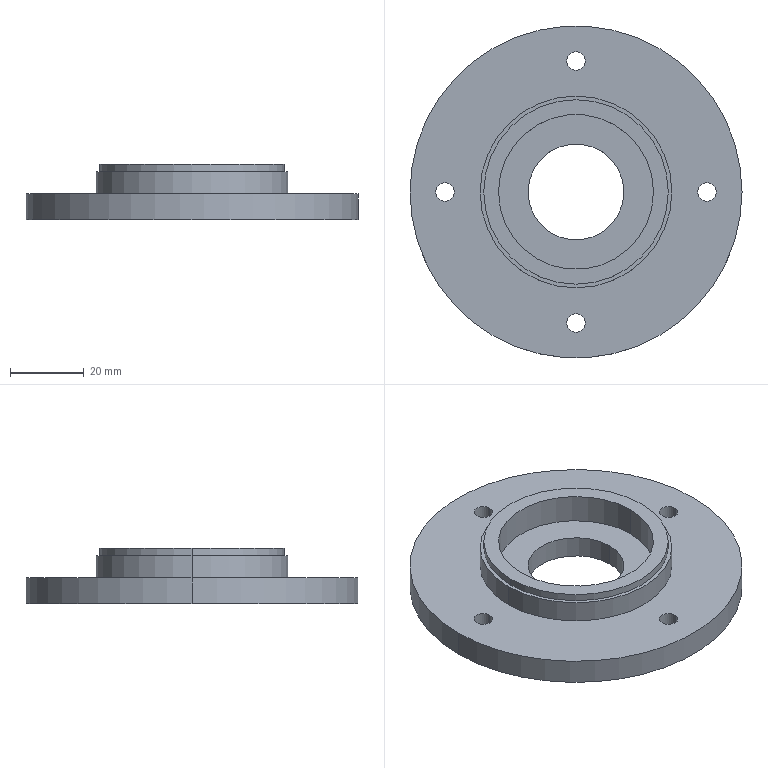Part | SolidWorks | features BaseBody 1 | 1 solid | 28 faces | box 90 x 90 x 15 mm | volume 44792 mm3 | cylinder 18 | plane 6 | torus 4 | commonest cylinder face diameters 5 x8 26 x2 42 x2 50 x2 52 x2 90 x2
STEP:
#1=CARTESIAN_POINT('',(-22.5,0.,0.5));
#2=VERTEX_POINT('',#1);
#3=CARTESIAN_POINT('',(22.5,0.,0.5));
#4=VERTEX_POINT('',#3);
#5=CARTESIAN_POINT('',(0.,0.,0.5));
#6=DIRECTION('',(0.,0.,1.));
#7=DIRECTION('',(1.,0.,0.));
#8=AXIS2_PLACEMENT_3D('',#5,#6,#7);
#9=CIRCLE('',#8,22.5);
#10=EDGE_CURVE('',#2,#4,#9,.T.);
#11=ORIENTED_EDGE('',*,*,#10,.F.);
#12=CARTESIAN_POINT('',(-22.,0.,1.));
#13=VERTEX_POINT('',#12);
#14=CARTESIAN_POINT('',(-22.,0.,0.5));
#15=DIRECTION('',(0.,1.,0.));
#16=DIRECTION('',(-1.,0.,0.));
#17=AXIS2_PLACEMENT_3D('',#14,#15,#16);
#18=CIRCLE('',#17,0.5);
#19=EDGE_CURVE('',#2,#13,#18,.T.);
#20=ORIENTED_EDGE('',*,*,#19,.T.);
#21=CARTESIAN_POINT('',(22.,0.,1.));
#22=VERTEX_POINT('',#21);
#23=CARTESIAN_POINT('',(0.,0.,1.));
#24=DIRECTION('',(0.,0.,1.));
#25=DIRECTION('',(1.,0.,0.));
#26=AXIS2_PLACEMENT_3D('',#23,#24,#25);
#27=CIRCLE('',#26,22.);
#28=EDGE_CURVE('',#13,#22,#27,.T.);
#29=ORIENTED_EDGE('',*,*,#28,.T.);
#30=CARTESIAN_POINT('',(22.,0.,0.5));
#31=DIRECTION('',(0.,-1.,0.));
#32=DIRECTION('',(0.,0.,-1.));
#33=AXIS2_PLACEMENT_3D('',#30,#31,#32);
#34=CIRCLE('',#33,0.5);
#35=EDGE_CURVE('',#4,#22,#34,.T.);
#36=ORIENTED_EDGE('',*,*,#35,.F.);
#37=EDGE_LOOP('',(#11,#20,#29,#36));
#38=FACE_OUTER_BOUND('',#37,.T.);
#39=CARTESIAN_POINT('',(0.,0.,0.5));
#40=DIRECTION('',(0.,0.,1.));
#41=DIRECTION('',(1.,0.,0.));
#42=AXIS2_PLACEMENT_3D('',#39,#40,#41);
#43=TOROIDAL_SURFACE('',#42,22.,0.5);
#44=ADVANCED_FACE('',(#38),#43,.F.);
#45=CARTESIAN_POINT('',(0.,0.,0.5));
#46=DIRECTION('',(0.,0.,1.));
#47=DIRECTION('',(1.,0.,0.));
#48=AXIS2_PLACEMENT_3D('',#45,#46,#47);
#49=CIRCLE('',#48,22.5);
#50=EDGE_CURVE('',#4,#2,#49,.T.);
#51=ORIENTED_EDGE('',*,*,#50,.T.);
#52=CARTESIAN_POINT('',(-23.,0.,0.));
#53=VERTEX_POINT('',#52);
#54=CARTESIAN_POINT('',(-23.,0.,0.5));
#55=DIRECTION('',(0.,1.,0.));
#56=DIRECTION('',(-1.,0.,0.));
#57=AXIS2_PLACEMENT_3D('',#54,#55,#56);
#58=CIRCLE('',#57,0.5);
#59=EDGE_CURVE('',#2,#53,#58,.T.);
#60=ORIENTED_EDGE('',*,*,#59,.T.);
#61=CARTESIAN_POINT('',(23.,0.,0.));
#62=VERTEX_POINT('',#61);
#63=CARTESIAN_POINT('',(0.,0.,0.));
#64=DIRECTION('',(0.,0.,-1.));
#65=DIRECTION('',(1.,0.,0.));
#66=AXIS2_PLACEMENT_3D('',#63,#64,#65);
#67=CIRCLE('',#66,23.);
#68=EDGE_CURVE('',#53,#62,#67,.T.);
#69=ORIENTED_EDGE('',*,*,#68,.T.);
#70=CARTESIAN_POINT('',(23.,0.,0.5));
#71=DIRECTION('',(0.,-1.,0.));
#72=DIRECTION('',(0.,0.,-1.));
#73=AXIS2_PLACEMENT_3D('',#70,#71,#72);
#74=CIRCLE('',#73,0.5);
#75=EDGE_CURVE('',#4,#62,#74,.T.);
#76=ORIENTED_EDGE('',*,*,#75,.F.);
#77=EDGE_LOOP('',(#51,#60,#69,#76));
#78=FACE_OUTER_BOUND('',#77,.T.);
#79=CARTESIAN_POINT('',(0.,0.,0.5));
#80=DIRECTION('',(0.,0.,1.));
#81=DIRECTION('',(1.,0.,0.));
#82=AXIS2_PLACEMENT_3D('',#79,#80,#81);
#83=TOROIDAL_SURFACE('',#82,23.,0.5);
#84=ADVANCED_FACE('',(#78),#83,.T.);
#85=CARTESIAN_POINT('',(33.,0.,7.));
#86=VERTEX_POINT('',#85);
#87=CARTESIAN_POINT('',(38.,0.,7.));
#88=VERTEX_POINT('',#87);
#89=CARTESIAN_POINT('',(35.5,0.,7.));
#90=DIRECTION('',(0.,0.,-1.));
#91=DIRECTION('',(1.,0.,0.));
#92=AXIS2_PLACEMENT_3D('',#89,#90,#91);
#93=CIRCLE('',#92,2.5);
#94=EDGE_CURVE('',#86,#88,#93,.T.);
#95=ORIENTED_EDGE('',*,*,#94,.F.);
#96=CARTESIAN_POINT('',(33.,0.,0.));
#97=VERTEX_POINT('',#96);
#98=CARTESIAN_POINT('',(33.,0.,0.));
#99=DIRECTION('',(0.,0.,-1.));
#100=VECTOR('',#99,1000.);
#101=LINE('',#98,#100);
#102=EDGE_CURVE('',#86,#97,#101,.T.);
#103=ORIENTED_EDGE('',*,*,#102,.T.);
#104=CARTESIAN_POINT('',(38.,0.,0.));
#105=VERTEX_POINT('',#104);
#106=CARTESIAN_POINT('',(35.5,0.,0.));
#107=DIRECTION('',(0.,0.,1.));
#108=DIRECTION('',(1.,0.,0.));
#109=AXIS2_PLACEMENT_3D('',#106,#107,#108);
#110=CIRCLE('',#109,2.5);
#111=EDGE_CURVE('',#105,#97,#110,.T.);
#112=ORIENTED_EDGE('',*,*,#111,.F.);
#113=CARTESIAN_POINT('',(38.,0.,0.));
#114=DIRECTION('',(0.,0.,-1.));
#115=VECTOR('',#114,1000.);
#116=LINE('',#113,#115);
#117=EDGE_CURVE('',#88,#105,#116,.T.);
#118=ORIENTED_EDGE('',*,*,#117,.F.);
#119=EDGE_LOOP('',(#95,#103,#112,#118));
#120=FACE_OUTER_BOUND('',#119,.T.);
#121=CARTESIAN_POINT('',(35.5,0.,0.));
#122=DIRECTION('',(0.,0.,-1.));
#123=DIRECTION('',(1.,0.,0.));
#124=AXIS2_PLACEMENT_3D('',#121,#122,#123);
#125=CYLINDRICAL_SURFACE('',#124,2.5);
#126=ADVANCED_FACE('',(#120),#125,.F.);
#127=CARTESIAN_POINT('',(-2.5,-35.5,7.));
#128=VERTEX_POINT('',#127);
#129=CARTESIAN_POINT('',(2.5,-35.5,7.));
#130=VERTEX_POINT('',#129);
#131=CARTESIAN_POINT('',(0.,-35.5,7.));
#132=DIRECTION('',(0.,0.,-1.));
#133=DIRECTION('',(1.,0.,0.));
#134=AXIS2_PLACEMENT_3D('',#131,#132,#133);
#135=CIRCLE('',#134,2.5);
#136=EDGE_CURVE('',#128,#130,#135,.T.);
#137=ORIENTED_EDGE('',*,*,#136,.F.);
#138=CARTESIAN_POINT('',(-2.5,-35.5,0.));
#139=VERTEX_POINT('',#138);
#140=CARTESIAN_POINT('',(-2.5,-35.5,0.));
#141=DIRECTION('',(0.,0.,-1.));
#142=VECTOR('',#141,1000.);
#143=LINE('',#140,#142);
#144=EDGE_CURVE('',#128,#139,#143,.T.);
#145=ORIENTED_EDGE('',*,*,#144,.T.);
#146=CARTESIAN_POINT('',(2.5,-35.5,0.));
#147=VERTEX_POINT('',#146);
#148=CARTESIAN_POINT('',(0.,-35.5,0.));
#149=DIRECTION('',(0.,0.,1.));
#150=DIRECTION('',(1.,0.,0.));
#151=AXIS2_PLACEMENT_3D('',#148,#149,#150);
#152=CIRCLE('',#151,2.5);
#153=EDGE_CURVE('',#147,#139,#152,.T.);
#154=ORIENTED_EDGE('',*,*,#153,.F.);
#155=CARTESIAN_POINT('',(2.5,-35.5,0.));
#156=DIRECTION('',(0.,0.,-1.));
#157=VECTOR('',#156,1000.);
#158=LINE('',#155,#157);
#159=EDGE_CURVE('',#130,#147,#158,.T.);
#160=ORIENTED_EDGE('',*,*,#159,.F.);
#161=EDGE_LOOP('',(#137,#145,#154,#160));
#162=FACE_OUTER_BOUND('',#161,.T.);
#163=CARTESIAN_POINT('',(0.,-35.5,0.));
#164=DIRECTION('',(0.,0.,-1.));
#165=DIRECTION('',(1.,0.,0.));
#166=AXIS2_PLACEMENT_3D('',#163,#164,#165);
#167=CYLINDRICAL_SURFACE('',#166,2.5);
#168=ADVANCED_FACE('',(#162),#167,.F.);
#169=CARTESIAN_POINT('',(-38.,0.,7.));
#170=VERTEX_POINT('',#169);
#171=CARTESIAN_POINT('',(-33.,0.,7.));
#172=VERTEX_POINT('',#171);
#173=CARTESIAN_POINT('',(-35.5,0.,7.));
#174=DIRECTION('',(0.,0.,-1.));
#175=DIRECTION('',(1.,0.,0.));
#176=AXIS2_PLACEMENT_3D('',#173,#174,#175);
#177=CIRCLE('',#176,2.5);
#178=EDGE_CURVE('',#170,#172,#177,.T.);
#179=ORIENTED_EDGE('',*,*,#178,.F.);
#180=CARTESIAN_POINT('',(-38.,0.,0.));
#181=VERTEX_POINT('',#180);
#182=CARTESIAN_POINT('',(-38.,0.,0.));
#183=DIRECTION('',(0.,0.,-1.));
#184=VECTOR('',#183,1000.);
#185=LINE('',#182,#184);
#186=EDGE_CURVE('',#170,#181,#185,.T.);
#187=ORIENTED_EDGE('',*,*,#186,.T.);
#188=CARTESIAN_POINT('',(-33.,0.,0.));
#189=VERTEX_POINT('',#188);
#190=CARTESIAN_POINT('',(-35.5,0.,0.));
#191=DIRECTION('',(0.,0.,1.));
#192=DIRECTION('',(1.,0.,0.));
#193=AXIS2_PLACEMENT_3D('',#190,#191,#192);
#194=CIRCLE('',#193,2.5);
#195=EDGE_CURVE('',#189,#181,#194,.T.);
#196=ORIENTED_EDGE('',*,*,#195,.F.);
#197=CARTESIAN_POINT('',(-33.,0.,0.));
#198=DIRECTION('',(0.,0.,-1.));
#199=VECTOR('',#198,1000.);
#200=LINE('',#197,#199);
#201=EDGE_CURVE('',#172,#189,#200,.T.);
#202=ORIENTED_EDGE('',*,*,#201,.F.);
#203=EDGE_LOOP('',(#179,#187,#196,#202));
#204=FACE_OUTER_BOUND('',#203,.T.);
#205=CARTESIAN_POINT('',(-35.5,0.,0.));
#206=DIRECTION('',(0.,0.,-1.));
#207=DIRECTION('',(1.,0.,0.));
#208=AXIS2_PLACEMENT_3D('',#205,#206,#207);
#209=CYLINDRICAL_SURFACE('',#208,2.5);
#210=ADVANCED_FACE('',(#204),#209,.F.);
#211=CARTESIAN_POINT('',(-2.5,35.5,7.));
#212=VERTEX_POINT('',#211);
#213=CARTESIAN_POINT('',(2.5,35.5,7.));
#214=VERTEX_POINT('',#213);
#215=CARTESIAN_POINT('',(0.,35.5,7.));
#216=DIRECTION('',(0.,0.,-1.));
#217=DIRECTION('',(1.,0.,0.));
#218=AXIS2_PLACEMENT_3D('',#215,#216,#217);
#219=CIRCLE('',#218,2.5);
#220=EDGE_CURVE('',#212,#214,#219,.T.);
#221=ORIENTED_EDGE('',*,*,#220,.F.);
#222=CARTESIAN_POINT('',(-2.5,35.5,0.));
#223=VERTEX_POINT('',#222);
#224=CARTESIAN_POINT('',(-2.5,35.5,0.));
#225=DIRECTION('',(0.,0.,-1.));
#226=VECTOR('',#225,1000.);
#227=LINE('',#224,#226);
#228=EDGE_CURVE('',#212,#223,#227,.T.);
#229=ORIENTED_EDGE('',*,*,#228,.T.);
#230=CARTESIAN_POINT('',(2.5,35.5,0.));
#231=VERTEX_POINT('',#230);
#232=CARTESIAN_POINT('',(0.,35.5,0.));
#233=DIRECTION('',(0.,0.,1.));
#234=DIRECTION('',(1.,0.,0.));
#235=AXIS2_PLACEMENT_3D('',#232,#233,#234);
#236=CIRCLE('',#235,2.5);
#237=EDGE_CURVE('',#231,#223,#236,.T.);
#238=ORIENTED_EDGE('',*,*,#237,.F.);
#239=CARTESIAN_POINT('',(2.5,35.5,0.));
#240=DIRECTION('',(0.,0.,-1.));
#241=VECTOR('',#240,1000.);
#242=LINE('',#239,#241);
#243=EDGE_CURVE('',#214,#231,#242,.T.);
#244=ORIENTED_EDGE('',*,*,#243,.F.);
#245=EDGE_LOOP('',(#221,#229,#238,#244));
#246=FACE_OUTER_BOUND('',#245,.T.);
#247=CARTESIAN_POINT('',(0.,35.5,0.));
#248=DIRECTION('',(0.,0.,-1.));
#249=DIRECTION('',(1.,0.,0.));
#250=AXIS2_PLACEMENT_3D('',#247,#248,#249);
#251=CYLINDRICAL_SURFACE('',#250,2.5);
#252=ADVANCED_FACE('',(#246),#251,.F.);
#253=CARTESIAN_POINT('',(-13.,0.,1.));
#254=VERTEX_POINT('',#253);
#255=CARTESIAN_POINT('',(13.,0.,1.));
#256=VERTEX_POINT('',#255);
#257=CARTESIAN_POINT('',(0.,0.,1.));
#258=DIRECTION('',(0.,0.,-1.));
#259=DIRECTION('',(-1.,0.,0.));
#260=AXIS2_PLACEMENT_3D('',#257,#258,#259);
#261=CIRCLE('',#260,13.);
#262=EDGE_CURVE('',#254,#256,#261,.T.);
#263=ORIENTED_EDGE('',*,*,#262,.T.);
#264=CARTESIAN_POINT('',(13.,0.,7.));
#265=VERTEX_POINT('',#264);
#266=CARTESIAN_POINT('',(13.,0.,7.));
#267=DIRECTION('',(0.,0.,1.));
#268=VECTOR('',#267,1000.);
#269=LINE('',#266,#268);
#270=EDGE_CURVE('',#256,#265,#269,.T.);
#271=ORIENTED_EDGE('',*,*,#270,.T.);
#272=CARTESIAN_POINT('',(-13.,0.,7.));
#273=VERTEX_POINT('',#272);
#274=CARTESIAN_POINT('',(0.,0.,7.));
#275=DIRECTION('',(0.,0.,-1.));
#276=DIRECTION('',(-1.,0.,0.));
#277=AXIS2_PLACEMENT_3D('',#274,#275,#276);
#278=CIRCLE('',#277,13.);
#279=EDGE_CURVE('',#273,#265,#278,.T.);
#280=ORIENTED_EDGE('',*,*,#279,.F.);
#281=CARTESIAN_POINT('',(-13.,0.,7.));
#282=DIRECTION('',(0.,0.,1.));
#283=VECTOR('',#282,1000.);
#284=LINE('',#281,#283);
#285=EDGE_CURVE('',#254,#273,#284,.T.);
#286=ORIENTED_EDGE('',*,*,#285,.F.);
#287=EDGE_LOOP('',(#263,#271,#280,#286));
#288=FACE_OUTER_BOUND('',#287,.T.);
#289=CARTESIAN_POINT('',(0.,0.,7.));
#290=DIRECTION('',(0.,0.,1.));
#291=DIRECTION('',(-1.,0.,0.));
#292=AXIS2_PLACEMENT_3D('',#289,#290,#291);
#293=CYLINDRICAL_SURFACE('',#292,13.);
#294=ADVANCED_FACE('',(#288),#293,.F.);
#295=CARTESIAN_POINT('',(-25.,0.,13.));
#296=VERTEX_POINT('',#295);
#297=CARTESIAN_POINT('',(25.,0.,13.));
#298=VERTEX_POINT('',#297);
#299=CARTESIAN_POINT('',(0.,0.,13.));
#300=DIRECTION('',(0.,0.,1.));
#301=DIRECTION('',(-1.,0.,0.));
#302=AXIS2_PLACEMENT_3D('',#299,#300,#301);
#303=CIRCLE('',#302,25.);
#304=EDGE_CURVE('',#296,#298,#303,.T.);
#305=ORIENTED_EDGE('',*,*,#304,.T.);
#306=CARTESIAN_POINT('',(25.,0.,15.));
#307=VERTEX_POINT('',#306);
#308=CARTESIAN_POINT('',(25.,0.,15.));
#309=DIRECTION('',(0.,0.,1.));
#310=VECTOR('',#309,1000.);
#311=LINE('',#308,#310);
#312=EDGE_CURVE('',#298,#307,#311,.T.);
#313=ORIENTED_EDGE('',*,*,#312,.T.);
#314=CARTESIAN_POINT('',(-25.,0.,15.));
#315=VERTEX_POINT('',#314);
#316=CARTESIAN_POINT('',(0.,0.,15.));
#317=DIRECTION('',(0.,0.,1.));
#318=DIRECTION('',(-1.,0.,0.));
#319=AXIS2_PLACEMENT_3D('',#316,#317,#318);
#320=CIRCLE('',#319,25.);
#321=EDGE_CURVE('',#315,#307,#320,.T.);
#322=ORIENTED_EDGE('',*,*,#321,.F.);
#323=CARTESIAN_POINT('',(-25.,0.,15.));
#324=DIRECTION('',(0.,0.,1.));
#325=VECTOR('',#324,1000.);
#326=LINE('',#323,#325);
#327=EDGE_CURVE('',#296,#315,#326,.T.);
#328=ORIENTED_EDGE('',*,*,#327,.F.);
#329=EDGE_LOOP('',(#305,#313,#322,#328));
#330=FACE_OUTER_BOUND('',#329,.T.);
#331=CARTESIAN_POINT('',(0.,0.,15.));
#332=DIRECTION('',(0.,0.,1.));
#333=DIRECTION('',(-1.,0.,0.));
#334=AXIS2_PLACEMENT_3D('',#331,#332,#333);
#335=CYLINDRICAL_SURFACE('',#334,25.);
#336=ADVANCED_FACE('',(#330),#335,.T.);
#337=CARTESIAN_POINT('',(21.,0.,15.));
#338=VERTEX_POINT('',#337);
#339=CARTESIAN_POINT('',(-21.,0.,15.));
#340=VERTEX_POINT('',#339);
#341=CARTESIAN_POINT('',(0.,0.,15.));
#342=DIRECTION('',(0.,0.,-1.));
#343=DIRECTION('',(-1.,0.,0.));
#344=AXIS2_PLACEMENT_3D('',#341,#342,#343);
#345=CIRCLE('',#344,21.);
#346=EDGE_CURVE('',#338,#340,#345,.T.);
#347=ORIENTED_EDGE('',*,*,#346,.F.);
#348=CARTESIAN_POINT('',(21.,0.,7.));
#349=VERTEX_POINT('',#348);
#350=CARTESIAN_POINT('',(21.,0.,7.));
#351=DIRECTION('',(0.,0.,-1.));
#352=VECTOR('',#351,1000.);
#353=LINE('',#350,#352);
#354=EDGE_CURVE('',#338,#349,#353,.T.);
#355=ORIENTED_EDGE('',*,*,#354,.T.);
#356=CARTESIAN_POINT('',(-21.,0.,7.));
#357=VERTEX_POINT('',#356);
#358=CARTESIAN_POINT('',(0.,0.,7.));
#359=DIRECTION('',(0.,0.,1.));
#360=DIRECTION('',(-1.,0.,0.));
#361=AXIS2_PLACEMENT_3D('',#358,#359,#360);
#362=CIRCLE('',#361,21.);
#363=EDGE_CURVE('',#357,#349,#362,.T.);
#364=ORIENTED_EDGE('',*,*,#363,.F.);
#365=CARTESIAN_POINT('',(-21.,0.,7.));
#366=DIRECTION('',(0.,0.,-1.));
#367=VECTOR('',#366,1000.);
#368=LINE('',#365,#367);
#369=EDGE_CURVE('',#340,#357,#368,.T.);
#370=ORIENTED_EDGE('',*,*,#369,.F.);
#371=EDGE_LOOP('',(#347,#355,#364,#370));
#372=FACE_OUTER_BOUND('',#371,.T.);
#373=CARTESIAN_POINT('',(0.,0.,7.));
#374=DIRECTION('',(0.,0.,-1.));
#375=DIRECTION('',(-1.,0.,0.));
#376=AXIS2_PLACEMENT_3D('',#373,#374,#375);
#377=CYLINDRICAL_SURFACE('',#376,21.);
#378=ADVANCED_FACE('',(#372),#377,.F.);
#379=CARTESIAN_POINT('',(-26.,0.,13.));
#380=VERTEX_POINT('',#379);
#381=CARTESIAN_POINT('',(26.,0.,13.));
#382=VERTEX_POINT('',#381);
#383=CARTESIAN_POINT('',(0.,0.,13.));
#384=DIRECTION('',(0.,0.,-1.));
#385=DIRECTION('',(-1.,0.,0.));
#386=AXIS2_PLACEMENT_3D('',#383,#384,#385);
#387=CIRCLE('',#386,26.);
#388=EDGE_CURVE('',#380,#382,#387,.T.);
#389=ORIENTED_EDGE('',*,*,#388,.T.);
#390=CARTESIAN_POINT('',(26.,0.,7.));
#391=VERTEX_POINT('',#390);
#392=CARTESIAN_POINT('',(26.,0.,7.));
#393=DIRECTION('',(0.,0.,-1.));
#394=VECTOR('',#393,1000.);
#395=LINE('',#392,#394);
#396=EDGE_CURVE('',#382,#391,#395,.T.);
#397=ORIENTED_EDGE('',*,*,#396,.T.);
#398=CARTESIAN_POINT('',(-26.,0.,7.));
#399=VERTEX_POINT('',#398);
#400=CARTESIAN_POINT('',(0.,0.,7.));
#401=DIRECTION('',(0.,0.,-1.));
#402=DIRECTION('',(-1.,0.,0.));
#403=AXIS2_PLACEMENT_3D('',#400,#401,#402);
#404=CIRCLE('',#403,26.);
#405=EDGE_CURVE('',#399,#391,#404,.T.);
#406=ORIENTED_EDGE('',*,*,#405,.F.);
#407=CARTESIAN_POINT('',(-26.,0.,7.));
#408=DIRECTION('',(0.,0.,-1.));
#409=VECTOR('',#408,1000.);
#410=LINE('',#407,#409);
#411=EDGE_CURVE('',#380,#399,#410,.T.);
#412=ORIENTED_EDGE('',*,*,#411,.F.);
#413=EDGE_LOOP('',(#389,#397,#406,#412));
#414=FACE_OUTER_BOUND('',#413,.T.);
#415=CARTESIAN_POINT('',(0.,0.,7.));
#416=DIRECTION('',(0.,0.,-1.));
#417=DIRECTION('',(-1.,0.,0.));
#418=AXIS2_PLACEMENT_3D('',#415,#416,#417);
#419=CYLINDRICAL_SURFACE('',#418,26.);
#420=ADVANCED_FACE('',(#414),#419,.T.);
#421=CARTESIAN_POINT('',(45.,0.,7.));
#422=VERTEX_POINT('',#421);
#423=CARTESIAN_POINT('',(-45.,0.,7.));
#424=VERTEX_POINT('',#423);
#425=CARTESIAN_POINT('',(0.,0.,7.));
#426=DIRECTION('',(0.,0.,1.));
#427=DIRECTION('',(-1.,0.,0.));
#428=AXIS2_PLACEMENT_3D('',#425,#426,#427);
#429=CIRCLE('',#428,45.);
#430=EDGE_CURVE('',#422,#424,#429,.T.);
#431=ORIENTED_EDGE('',*,*,#430,.F.);
#432=CARTESIAN_POINT('',(45.,0.,0.));
#433=VERTEX_POINT('',#432);
#434=CARTESIAN_POINT('',(45.,0.,0.));
#435=DIRECTION('',(0.,0.,-1.));
#436=VECTOR('',#435,1000.);
#437=LINE('',#434,#436);
#438=EDGE_CURVE('',#422,#433,#437,.T.);
#439=ORIENTED_EDGE('',*,*,#438,.T.);
#440=CARTESIAN_POINT('',(-45.,0.,0.));
#441=VERTEX_POINT('',#440);
#442=CARTESIAN_POINT('',(0.,0.,0.));
#443=DIRECTION('',(0.,0.,-1.));
#444=DIRECTION('',(-1.,0.,0.));
#445=AXIS2_PLACEMENT_3D('',#442,#443,#444);
#446=CIRCLE('',#445,45.);
#447=EDGE_CURVE('',#441,#433,#446,.T.);
#448=ORIENTED_EDGE('',*,*,#447,.F.);
#449=CARTESIAN_POINT('',(-45.,0.,0.));
#450=DIRECTION('',(0.,0.,-1.));
#451=VECTOR('',#450,1000.);
#452=LINE('',#449,#451);
#453=EDGE_CURVE('',#424,#441,#452,.T.);
#454=ORIENTED_EDGE('',*,*,#453,.F.);
#455=EDGE_LOOP('',(#431,#439,#448,#454));
#456=FACE_OUTER_BOUND('',#455,.T.);
#457=CARTESIAN_POINT('',(0.,0.,0.));
#458=DIRECTION('',(0.,0.,-1.));
#459=DIRECTION('',(-1.,0.,0.));
#460=AXIS2_PLACEMENT_3D('',#457,#458,#459);
#461=CYLINDRICAL_SURFACE('',#460,45.);
#462=ADVANCED_FACE('',(#456),#461,.T.);
#463=ORIENTED_EDGE('',*,*,#262,.F.);
#464=CARTESIAN_POINT('',(0.,0.,1.));
#465=DIRECTION('',(0.,0.,-1.));
#466=DIRECTION('',(-1.,0.,0.));
#467=AXIS2_PLACEMENT_3D('',#464,#465,#466);
#468=CIRCLE('',#467,13.);
#469=EDGE_CURVE('',#256,#254,#468,.T.);
#470=ORIENTED_EDGE('',*,*,#469,.F.);
#471=EDGE_LOOP('',(#463,#470));
#472=FACE_BOUND('',#471,.T.);
#473=CARTESIAN_POINT('',(0.,0.,1.));
#474=DIRECTION('',(0.,0.,1.));
#475=DIRECTION('',(1.,0.,0.));
#476=AXIS2_PLACEMENT_3D('',#473,#474,#475);
#477=CIRCLE('',#476,22.);
#478=EDGE_CURVE('',#22,#13,#477,.T.);
#479=ORIENTED_EDGE('',*,*,#478,.F.);
#480=ORIENTED_EDGE('',*,*,#28,.F.);
#481=EDGE_LOOP('',(#479,#480));
#482=FACE_OUTER_BOUND('',#481,.T.);
#483=CARTESIAN_POINT('',(0.,0.,1.));
#484=DIRECTION('',(0.,0.,1.));
#485=DIRECTION('',(1.,0.,0.));
#486=AXIS2_PLACEMENT_3D('',#483,#484,#485);
#487=PLANE('',#486);
#488=ADVANCED_FACE('',(#472,#482),#487,.F.);
#489=ORIENTED_EDGE('',*,*,#237,.T.);
#490=CARTESIAN_POINT('',(0.,35.5,0.));
#491=DIRECTION('',(0.,0.,1.));
#492=DIRECTION('',(1.,0.,0.));
#493=AXIS2_PLACEMENT_3D('',#490,#491,#492);
#494=CIRCLE('',#493,2.5);
#495=EDGE_CURVE('',#223,#231,#494,.T.);
#496=ORIENTED_EDGE('',*,*,#495,.T.);
#497=EDGE_LOOP('',(#489,#496));
#498=FACE_BOUND('',#497,.T.);
#499=ORIENTED_EDGE('',*,*,#195,.T.);
#500=CARTESIAN_POINT('',(-35.5,0.,0.));
#501=DIRECTION('',(0.,0.,1.));
#502=DIRECTION('',(1.,0.,0.));
#503=AXIS2_PLACEMENT_3D('',#500,#501,#502);
#504=CIRCLE('',#503,2.5);
#505=EDGE_CURVE('',#181,#189,#504,.T.);
#506=ORIENTED_EDGE('',*,*,#505,.T.);
#507=EDGE_LOOP('',(#499,#506));
#508=FACE_BOUND('',#507,.T.);
#509=ORIENTED_EDGE('',*,*,#153,.T.);
#510=CARTESIAN_POINT('',(0.,-35.5,0.));
#511=DIRECTION('',(0.,0.,1.));
#512=DIRECTION('',(1.,0.,0.));
#513=AXIS2_PLACEMENT_3D('',#510,#511,#512);
#514=CIRCLE('',#513,2.5);
#515=EDGE_CURVE('',#139,#147,#514,.T.);
#516=ORIENTED_EDGE('',*,*,#515,.T.);
#517=EDGE_LOOP('',(#509,#516));
#518=FACE_BOUND('',#517,.T.);
#519=ORIENTED_EDGE('',*,*,#111,.T.);
#520=CARTESIAN_POINT('',(35.5,0.,0.));
#521=DIRECTION('',(0.,0.,1.));
#522=DIRECTION('',(1.,0.,0.));
#523=AXIS2_PLACEMENT_3D('',#520,#521,#522);
#524=CIRCLE('',#523,2.5);
#525=EDGE_CURVE('',#97,#105,#524,.T.);
#526=ORIENTED_EDGE('',*,*,#525,.T.);
#527=EDGE_LOOP('',(#519,#526));
#528=FACE_BOUND('',#527,.T.);
#529=CARTESIAN_POINT('',(0.,0.,0.));
#530=DIRECTION('',(0.,0.,-1.));
#531=DIRECTION('',(1.,0.,0.));
#532=AXIS2_PLACEMENT_3D('',#529,#530,#531);
#533=CIRCLE('',#532,23.);
#534=EDGE_CURVE('',#62,#53,#533,.T.);
#535=ORIENTED_EDGE('',*,*,#534,.F.);
#536=ORIENTED_EDGE('',*,*,#68,.F.);
#537=EDGE_LOOP('',(#535,#536));
#538=FACE_BOUND('',#537,.T.);
#539=ORIENTED_EDGE('',*,*,#447,.T.);
#540=CARTESIAN_POINT('',(0.,0.,0.));
#541=DIRECTION('',(0.,0.,-1.));
#542=DIRECTION('',(-1.,0.,0.));
#543=AXIS2_PLACEMENT_3D('',#540,#541,#542);
#544=CIRCLE('',#543,45.);
#545=EDGE_CURVE('',#433,#441,#544,.T.);
#546=ORIENTED_EDGE('',*,*,#545,.T.);
#547=EDGE_LOOP('',(#539,#546));
#548=FACE_OUTER_BOUND('',#547,.T.);
#549=CARTESIAN_POINT('',(0.,0.,0.));
#550=DIRECTION('',(0.,0.,1.));
#551=DIRECTION('',(1.,0.,0.));
#552=AXIS2_PLACEMENT_3D('',#549,#550,#551);
#553=PLANE('',#552);
#554=ADVANCED_FACE('',(#498,#508,#518,#528,#538,#548),#553,.F.);
#555=ORIENTED_EDGE('',*,*,#304,.F.);
#556=CARTESIAN_POINT('',(0.,0.,13.));
#557=DIRECTION('',(0.,0.,1.));
#558=DIRECTION('',(-1.,0.,0.));
#559=AXIS2_PLACEMENT_3D('',#556,#557,#558);
#560=CIRCLE('',#559,25.);
#561=EDGE_CURVE('',#298,#296,#560,.T.);
#562=ORIENTED_EDGE('',*,*,#561,.F.);
#563=EDGE_LOOP('',(#555,#562));
#564=FACE_BOUND('',#563,.T.);
#565=ORIENTED_EDGE('',*,*,#388,.F.);
#566=CARTESIAN_POINT('',(0.,0.,13.));
#567=DIRECTION('',(0.,0.,-1.));
#568=DIRECTION('',(-1.,0.,0.));
#569=AXIS2_PLACEMENT_3D('',#566,#567,#568);
#570=CIRCLE('',#569,26.);
#571=EDGE_CURVE('',#382,#380,#570,.T.);
#572=ORIENTED_EDGE('',*,*,#571,.F.);
#573=EDGE_LOOP('',(#565,#572));
#574=FACE_OUTER_BOUND('',#573,.T.);
#575=CARTESIAN_POINT('',(0.,0.,13.));
#576=DIRECTION('',(0.,0.,1.));
#577=DIRECTION('',(1.,0.,0.));
#578=AXIS2_PLACEMENT_3D('',#575,#576,#577);
#579=PLANE('',#578);
#580=ADVANCED_FACE('',(#564,#574),#579,.T.);
#581=CARTESIAN_POINT('',(0.,0.,15.));
#582=DIRECTION('',(0.,0.,-1.));
#583=DIRECTION('',(-1.,0.,0.));
#584=AXIS2_PLACEMENT_3D('',#581,#582,#583);
#585=CIRCLE('',#584,21.);
#586=EDGE_CURVE('',#340,#338,#585,.T.);
#587=ORIENTED_EDGE('',*,*,#586,.T.);
#588=ORIENTED_EDGE('',*,*,#346,.T.);
#589=EDGE_LOOP('',(#587,#588));
#590=FACE_BOUND('',#589,.T.);
#591=ORIENTED_EDGE('',*,*,#321,.T.);
#592=CARTESIAN_POINT('',(0.,0.,15.));
#593=DIRECTION('',(0.,0.,1.));
#594=DIRECTION('',(-1.,0.,0.));
#595=AXIS2_PLACEMENT_3D('',#592,#593,#594);
#596=CIRCLE('',#595,25.);
#597=EDGE_CURVE('',#307,#315,#596,.T.);
#598=ORIENTED_EDGE('',*,*,#597,.T.);
#599=EDGE_LOOP('',(#591,#598));
#600=FACE_OUTER_BOUND('',#599,.T.);
#601=CARTESIAN_POINT('',(0.,0.,15.));
#602=DIRECTION('',(0.,0.,1.));
#603=DIRECTION('',(1.,0.,0.));
#604=AXIS2_PLACEMENT_3D('',#601,#602,#603);
#605=PLANE('',#604);
#606=ADVANCED_FACE('',(#590,#600),#605,.T.);
#607=CARTESIAN_POINT('',(35.5,0.,7.));
#608=DIRECTION('',(0.,0.,-1.));
#609=DIRECTION('',(1.,0.,0.));
#610=AXIS2_PLACEMENT_3D('',#607,#608,#609);
#611=CIRCLE('',#610,2.5);
#612=EDGE_CURVE('',#88,#86,#611,.T.);
#613=ORIENTED_EDGE('',*,*,#612,.T.);
#614=ORIENTED_EDGE('',*,*,#94,.T.);
#615=EDGE_LOOP('',(#613,#614));
#616=FACE_BOUND('',#615,.T.);
#617=CARTESIAN_POINT('',(0.,-35.5,7.));
#618=DIRECTION('',(0.,0.,-1.));
#619=DIRECTION('',(1.,0.,0.));
#620=AXIS2_PLACEMENT_3D('',#617,#618,#619);
#621=CIRCLE('',#620,2.5);
#622=EDGE_CURVE('',#130,#128,#621,.T.);
#623=ORIENTED_EDGE('',*,*,#622,.T.);
#624=ORIENTED_EDGE('',*,*,#136,.T.);
#625=EDGE_LOOP('',(#623,#624));
#626=FACE_BOUND('',#625,.T.);
#627=CARTESIAN_POINT('',(-35.5,0.,7.));
#628=DIRECTION('',(0.,0.,-1.));
#629=DIRECTION('',(1.,0.,0.));
#630=AXIS2_PLACEMENT_3D('',#627,#628,#629);
#631=CIRCLE('',#630,2.5);
#632=EDGE_CURVE('',#172,#170,#631,.T.);
#633=ORIENTED_EDGE('',*,*,#632,.T.);
#634=ORIENTED_EDGE('',*,*,#178,.T.);
#635=EDGE_LOOP('',(#633,#634));
#636=FACE_BOUND('',#635,.T.);
#637=CARTESIAN_POINT('',(0.,35.5,7.));
#638=DIRECTION('',(0.,0.,-1.));
#639=DIRECTION('',(1.,0.,0.));
#640=AXIS2_PLACEMENT_3D('',#637,#638,#639);
#641=CIRCLE('',#640,2.5);
#642=EDGE_CURVE('',#214,#212,#641,.T.);
#643=ORIENTED_EDGE('',*,*,#642,.T.);
#644=ORIENTED_EDGE('',*,*,#220,.T.);
#645=EDGE_LOOP('',(#643,#644));
#646=FACE_BOUND('',#645,.T.);
#647=ORIENTED_EDGE('',*,*,#405,.T.);
#648=CARTESIAN_POINT('',(0.,0.,7.));
#649=DIRECTION('',(0.,0.,-1.));
#650=DIRECTION('',(-1.,0.,0.));
#651=AXIS2_PLACEMENT_3D('',#648,#649,#650);
#652=CIRCLE('',#651,26.);
#653=EDGE_CURVE('',#391,#399,#652,.T.);
#654=ORIENTED_EDGE('',*,*,#653,.T.);
#655=EDGE_LOOP('',(#647,#654));
#656=FACE_BOUND('',#655,.T.);
#657=CARTESIAN_POINT('',(0.,0.,7.));
#658=DIRECTION('',(0.,0.,1.));
#659=DIRECTION('',(-1.,0.,0.));
#660=AXIS2_PLACEMENT_3D('',#657,#658,#659);
#661=CIRCLE('',#660,45.);
#662=EDGE_CURVE('',#424,#422,#661,.T.);
#663=ORIENTED_EDGE('',*,*,#662,.T.);
#664=ORIENTED_EDGE('',*,*,#430,.T.);
#665=EDGE_LOOP('',(#663,#664));
#666=FACE_OUTER_BOUND('',#665,.T.);
#667=CARTESIAN_POINT('',(0.,0.,7.));
#668=DIRECTION('',(0.,0.,1.));
#669=DIRECTION('',(1.,0.,0.));
#670=AXIS2_PLACEMENT_3D('',#667,#668,#669);
#671=PLANE('',#670);
#672=ADVANCED_FACE('',(#616,#626,#636,#646,#656,#666),#671,.T.);
#673=ORIENTED_EDGE('',*,*,#279,.T.);
#674=CARTESIAN_POINT('',(0.,0.,7.));
#675=DIRECTION('',(0.,0.,-1.));
#676=DIRECTION('',(-1.,0.,0.));
#677=AXIS2_PLACEMENT_3D('',#674,#675,#676);
#678=CIRCLE('',#677,13.);
#679=EDGE_CURVE('',#265,#273,#678,.T.);
#680=ORIENTED_EDGE('',*,*,#679,.T.);
#681=EDGE_LOOP('',(#673,#680));
#682=FACE_BOUND('',#681,.T.);
#683=ORIENTED_EDGE('',*,*,#363,.T.);
#684=CARTESIAN_POINT('',(0.,0.,7.));
#685=DIRECTION('',(0.,0.,1.));
#686=DIRECTION('',(-1.,0.,0.));
#687=AXIS2_PLACEMENT_3D('',#684,#685,#686);
#688=CIRCLE('',#687,21.);
#689=EDGE_CURVE('',#349,#357,#688,.T.);
#690=ORIENTED_EDGE('',*,*,#689,.T.);
#691=EDGE_LOOP('',(#683,#690));
#692=FACE_OUTER_BOUND('',#691,.T.);
#693=CARTESIAN_POINT('',(0.,0.,7.));
#694=DIRECTION('',(0.,0.,1.));
#695=DIRECTION('',(1.,0.,0.));
#696=AXIS2_PLACEMENT_3D('',#693,#694,#695);
#697=PLANE('',#696);
#698=ADVANCED_FACE('',(#682,#692),#697,.T.);
#699=ORIENTED_EDGE('',*,*,#438,.F.);
#700=ORIENTED_EDGE('',*,*,#662,.F.);
#701=ORIENTED_EDGE('',*,*,#453,.T.);
#702=ORIENTED_EDGE('',*,*,#545,.F.);
#703=EDGE_LOOP('',(#699,#700,#701,#702));
#704=FACE_OUTER_BOUND('',#703,.T.);
#705=CARTESIAN_POINT('',(0.,0.,0.));
#706=DIRECTION('',(0.,0.,-1.));
#707=DIRECTION('',(-1.,0.,0.));
#708=AXIS2_PLACEMENT_3D('',#705,#706,#707);
#709=CYLINDRICAL_SURFACE('',#708,45.);
#710=ADVANCED_FACE('',(#704),#709,.T.);
#711=ORIENTED_EDGE('',*,*,#396,.F.);
#712=ORIENTED_EDGE('',*,*,#571,.T.);
#713=ORIENTED_EDGE('',*,*,#411,.T.);
#714=ORIENTED_EDGE('',*,*,#653,.F.);
#715=EDGE_LOOP('',(#711,#712,#713,#714));
#716=FACE_OUTER_BOUND('',#715,.T.);
#717=CARTESIAN_POINT('',(0.,0.,7.));
#718=DIRECTION('',(0.,0.,-1.));
#719=DIRECTION('',(-1.,0.,0.));
#720=AXIS2_PLACEMENT_3D('',#717,#718,#719);
#721=CYLINDRICAL_SURFACE('',#720,26.);
#722=ADVANCED_FACE('',(#716),#721,.T.);
#723=ORIENTED_EDGE('',*,*,#354,.F.);
#724=ORIENTED_EDGE('',*,*,#586,.F.);
#725=ORIENTED_EDGE('',*,*,#369,.T.);
#726=ORIENTED_EDGE('',*,*,#689,.F.);
#727=EDGE_LOOP('',(#723,#724,#725,#726));
#728=FACE_OUTER_BOUND('',#727,.T.);
#729=CARTESIAN_POINT('',(0.,0.,7.));
#730=DIRECTION('',(0.,0.,-1.));
#731=DIRECTION('',(-1.,0.,0.));
#732=AXIS2_PLACEMENT_3D('',#729,#730,#731);
#733=CYLINDRICAL_SURFACE('',#732,21.);
#734=ADVANCED_FACE('',(#728),#733,.F.);
#735=ORIENTED_EDGE('',*,*,#312,.F.);
#736=ORIENTED_EDGE('',*,*,#561,.T.);
#737=ORIENTED_EDGE('',*,*,#327,.T.);
#738=ORIENTED_EDGE('',*,*,#597,.F.);
#739=EDGE_LOOP('',(#735,#736,#737,#738));
#740=FACE_OUTER_BOUND('',#739,.T.);
#741=CARTESIAN_POINT('',(0.,0.,15.));
#742=DIRECTION('',(0.,0.,1.));
#743=DIRECTION('',(-1.,0.,0.));
#744=AXIS2_PLACEMENT_3D('',#741,#742,#743);
#745=CYLINDRICAL_SURFACE('',#744,25.);
#746=ADVANCED_FACE('',(#740),#745,.T.);
#747=ORIENTED_EDGE('',*,*,#270,.F.);
#748=ORIENTED_EDGE('',*,*,#469,.T.);
#749=ORIENTED_EDGE('',*,*,#285,.T.);
#750=ORIENTED_EDGE('',*,*,#679,.F.);
#751=EDGE_LOOP('',(#747,#748,#749,#750));
#752=FACE_OUTER_BOUND('',#751,.T.);
#753=CARTESIAN_POINT('',(0.,0.,7.));
#754=DIRECTION('',(0.,0.,1.));
#755=DIRECTION('',(-1.,0.,0.));
#756=AXIS2_PLACEMENT_3D('',#753,#754,#755);
#757=CYLINDRICAL_SURFACE('',#756,13.);
#758=ADVANCED_FACE('',(#752),#757,.F.);
#759=ORIENTED_EDGE('',*,*,#228,.F.);
#760=ORIENTED_EDGE('',*,*,#642,.F.);
#761=ORIENTED_EDGE('',*,*,#243,.T.);
#762=ORIENTED_EDGE('',*,*,#495,.F.);
#763=EDGE_LOOP('',(#759,#760,#761,#762));
#764=FACE_OUTER_BOUND('',#763,.T.);
#765=CARTESIAN_POINT('',(0.,35.5,0.));
#766=DIRECTION('',(0.,0.,-1.));
#767=DIRECTION('',(1.,0.,0.));
#768=AXIS2_PLACEMENT_3D('',#765,#766,#767);
#769=CYLINDRICAL_SURFACE('',#768,2.5);
#770=ADVANCED_FACE('',(#764),#769,.F.);
#771=ORIENTED_EDGE('',*,*,#186,.F.);
#772=ORIENTED_EDGE('',*,*,#632,.F.);
#773=ORIENTED_EDGE('',*,*,#201,.T.);
#774=ORIENTED_EDGE('',*,*,#505,.F.);
#775=EDGE_LOOP('',(#771,#772,#773,#774));
#776=FACE_OUTER_BOUND('',#775,.T.);
#777=CARTESIAN_POINT('',(-35.5,0.,0.));
#778=DIRECTION('',(0.,0.,-1.));
#779=DIRECTION('',(1.,0.,0.));
#780=AXIS2_PLACEMENT_3D('',#777,#778,#779);
#781=CYLINDRICAL_SURFACE('',#780,2.5);
#782=ADVANCED_FACE('',(#776),#781,.F.);
#783=ORIENTED_EDGE('',*,*,#144,.F.);
#784=ORIENTED_EDGE('',*,*,#622,.F.);
#785=ORIENTED_EDGE('',*,*,#159,.T.);
#786=ORIENTED_EDGE('',*,*,#515,.F.);
#787=EDGE_LOOP('',(#783,#784,#785,#786));
#788=FACE_OUTER_BOUND('',#787,.T.);
#789=CARTESIAN_POINT('',(0.,-35.5,0.));
#790=DIRECTION('',(0.,0.,-1.));
#791=DIRECTION('',(1.,0.,0.));
#792=AXIS2_PLACEMENT_3D('',#789,#790,#791);
#793=CYLINDRICAL_SURFACE('',#792,2.5);
#794=ADVANCED_FACE('',(#788),#793,.F.);
#795=ORIENTED_EDGE('',*,*,#102,.F.);
#796=ORIENTED_EDGE('',*,*,#612,.F.);
#797=ORIENTED_EDGE('',*,*,#117,.T.);
#798=ORIENTED_EDGE('',*,*,#525,.F.);
#799=EDGE_LOOP('',(#795,#796,#797,#798));
#800=FACE_OUTER_BOUND('',#799,.T.);
#801=CARTESIAN_POINT('',(35.5,0.,0.));
#802=DIRECTION('',(0.,0.,-1.));
#803=DIRECTION('',(1.,0.,0.));
#804=AXIS2_PLACEMENT_3D('',#801,#802,#803);
#805=CYLINDRICAL_SURFACE('',#804,2.5);
#806=ADVANCED_FACE('',(#800),#805,.F.);
#807=ORIENTED_EDGE('',*,*,#59,.F.);
#808=ORIENTED_EDGE('',*,*,#10,.T.);
#809=ORIENTED_EDGE('',*,*,#75,.T.);
#810=ORIENTED_EDGE('',*,*,#534,.T.);
#811=EDGE_LOOP('',(#807,#808,#809,#810));
#812=FACE_OUTER_BOUND('',#811,.T.);
#813=CARTESIAN_POINT('',(0.,0.,0.5));
#814=DIRECTION('',(0.,0.,1.));
#815=DIRECTION('',(1.,0.,0.));
#816=AXIS2_PLACEMENT_3D('',#813,#814,#815);
#817=TOROIDAL_SURFACE('',#816,23.,0.5);
#818=ADVANCED_FACE('',(#812),#817,.T.);
#819=ORIENTED_EDGE('',*,*,#19,.F.);
#820=ORIENTED_EDGE('',*,*,#50,.F.);
#821=ORIENTED_EDGE('',*,*,#35,.T.);
#822=ORIENTED_EDGE('',*,*,#478,.T.);
#823=EDGE_LOOP('',(#819,#820,#821,#822));
#824=FACE_OUTER_BOUND('',#823,.T.);
#825=CARTESIAN_POINT('',(0.,0.,0.5));
#826=DIRECTION('',(0.,0.,1.));
#827=DIRECTION('',(1.,0.,0.));
#828=AXIS2_PLACEMENT_3D('',#825,#826,#827);
#829=TOROIDAL_SURFACE('',#828,22.,0.5);
#830=ADVANCED_FACE('',(#824),#829,.F.);
#831=CLOSED_SHELL('',(#44,#84,#126,#168,#210,#252,#294,#336,#378,#420,#462,#488,#554,#580,#606,#672,#698,#710,#722,#734,#746,#758,#770,#782,#794,#806,#818,#830));
#832=MANIFOLD_SOLID_BREP('',#831);
#833=CARTESIAN_POINT('',(0.,0.,0.));
#834=DIRECTION('',(0.,0.,1.));
#835=DIRECTION('',(1.,0.,0.));
#836=AXIS2_PLACEMENT_3D('',#833,#834,#835);
#837=(LENGTH_UNIT()NAMED_UNIT(*)SI_UNIT(.MILLI.,.METRE.));
#838=UNCERTAINTY_MEASURE_WITH_UNIT(LENGTH_MEASURE(0.00001),#837,'','');
#839=(NAMED_UNIT(*)PLANE_ANGLE_UNIT()SI_UNIT($,.RADIAN.));
#840=(NAMED_UNIT(*)SI_UNIT($,.STERADIAN.)SOLID_ANGLE_UNIT());
#841=(GEOMETRIC_REPRESENTATION_CONTEXT(3)GLOBAL_UNCERTAINTY_ASSIGNED_CONTEXT((#838))GLOBAL_UNIT_ASSIGNED_CONTEXT((#837,#839,#840))REPRESENTATION_CONTEXT('',''));
#842=ADVANCED_BREP_SHAPE_REPRESENTATION('',(#832,#836),#841);